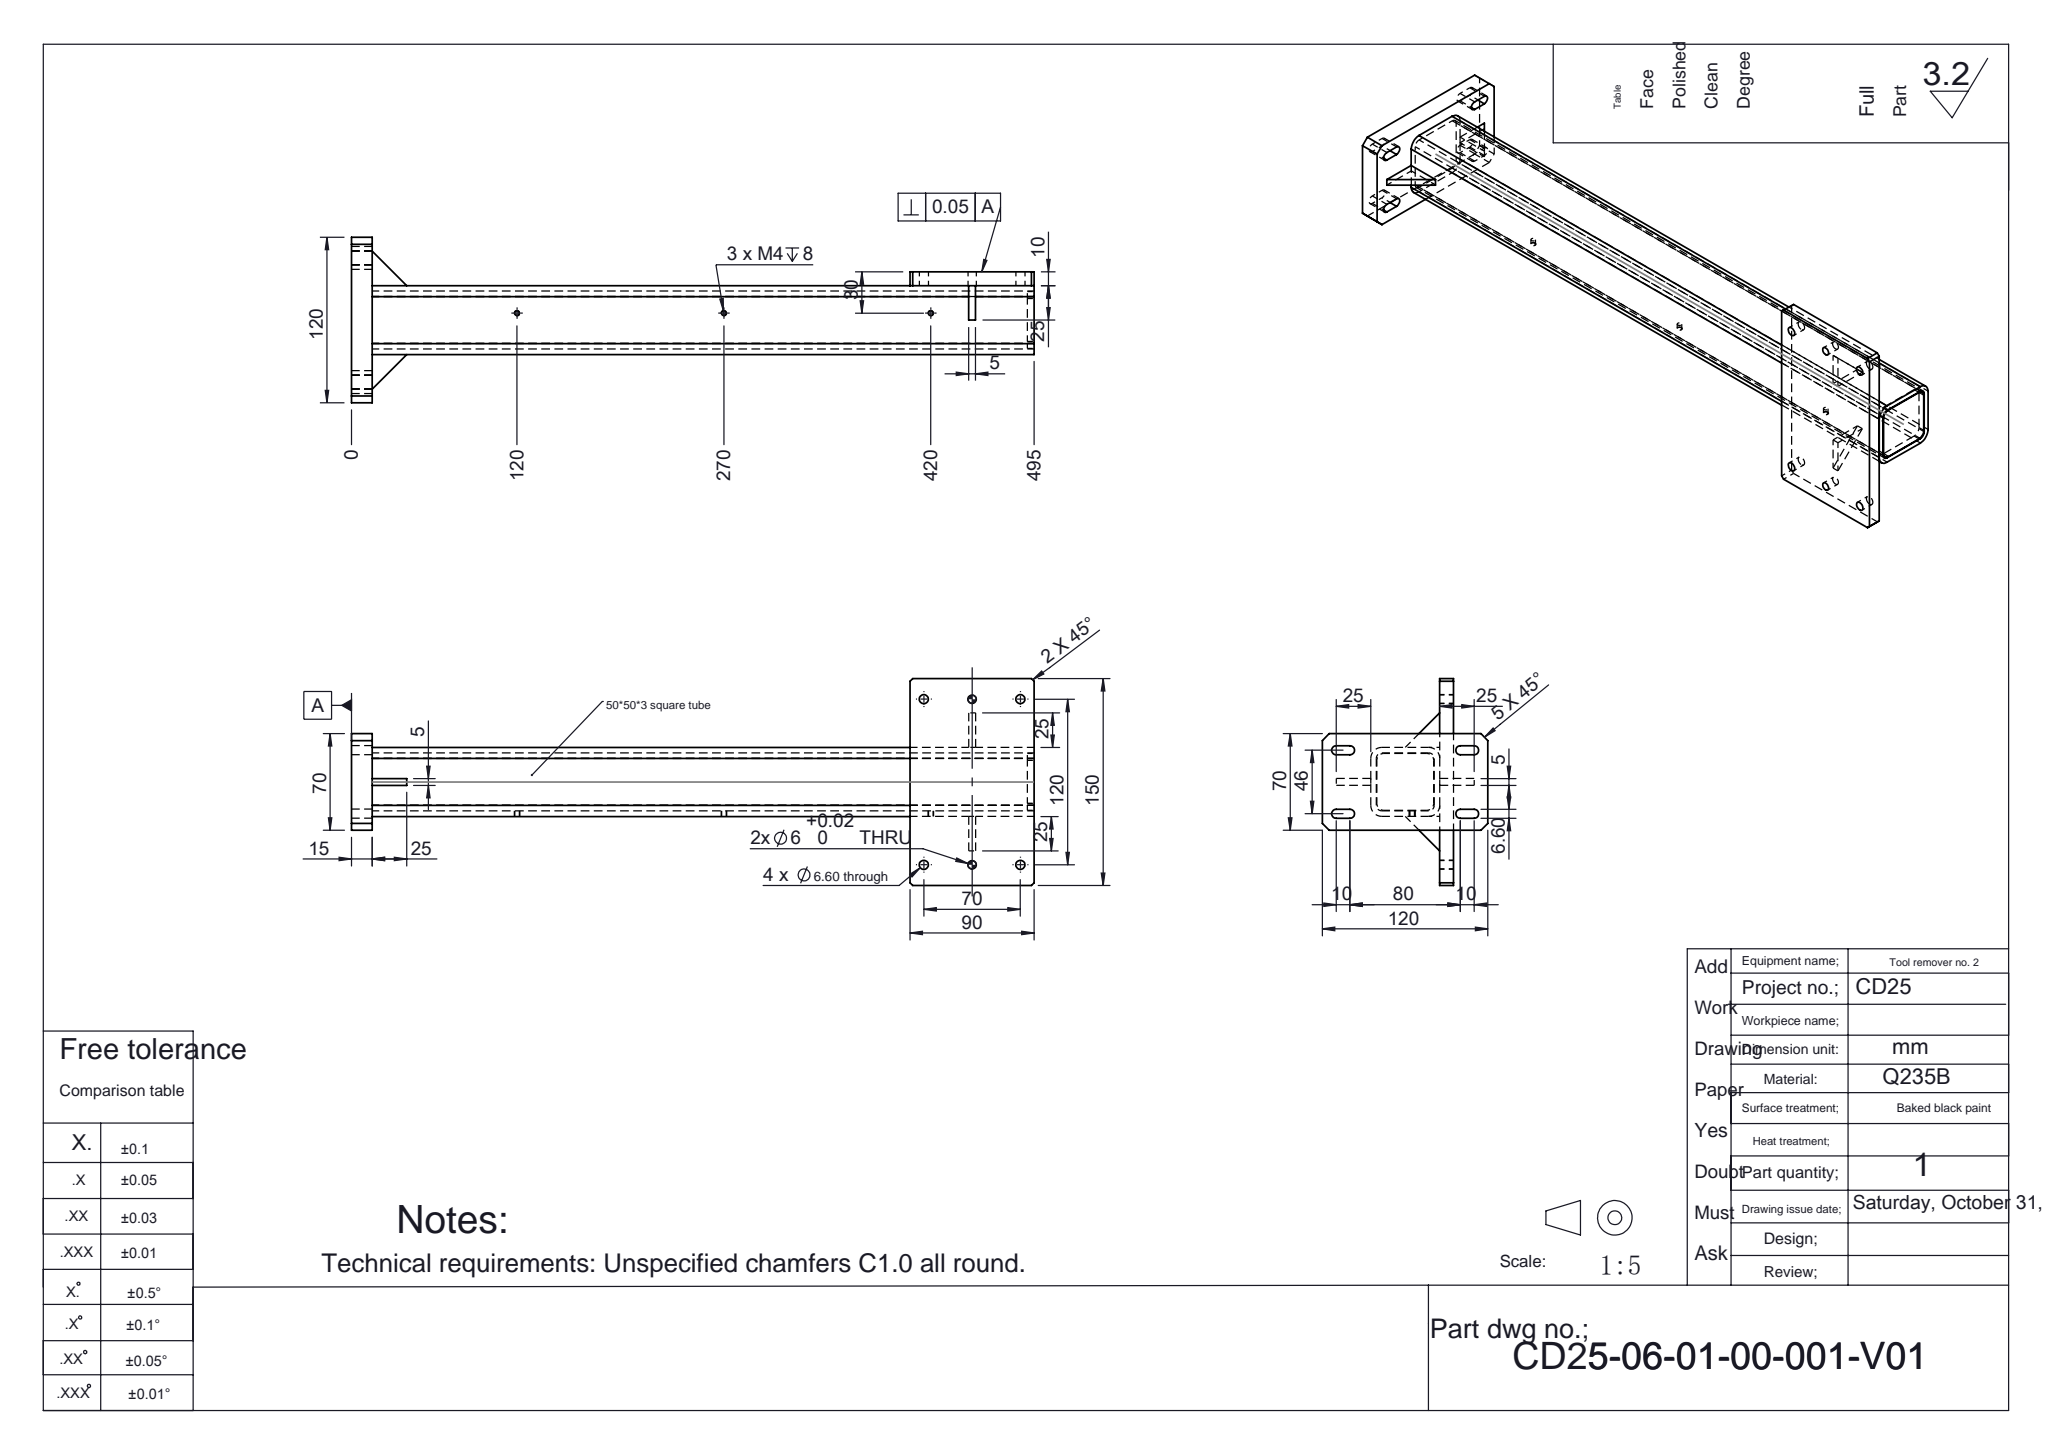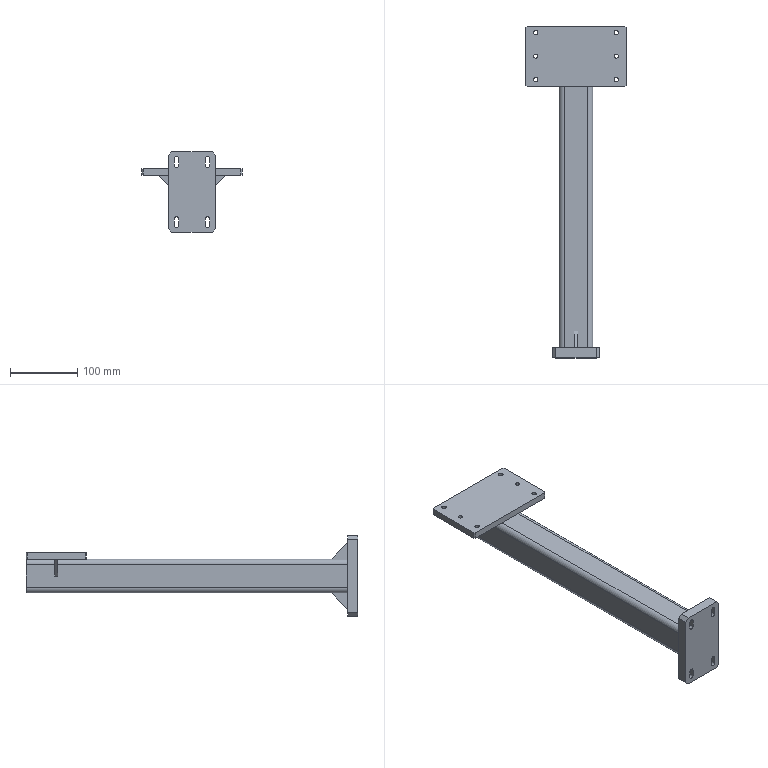Part | SolidWorks | features Gusset 4, HoleWzd 4, Chamfer 2, ICE 2, EndCap 1, WeldMemberFeat 1, WeldmentFeature 1 | 8 solids | 106 faces | box 150 x 495 x 120 mm | volume 600253 mm3 | plane 64 | cylinder 42 | commonest cylinder face diameters 6.6 x20 3.3 x6 6 x4 8 x4 10 x4 16 x4